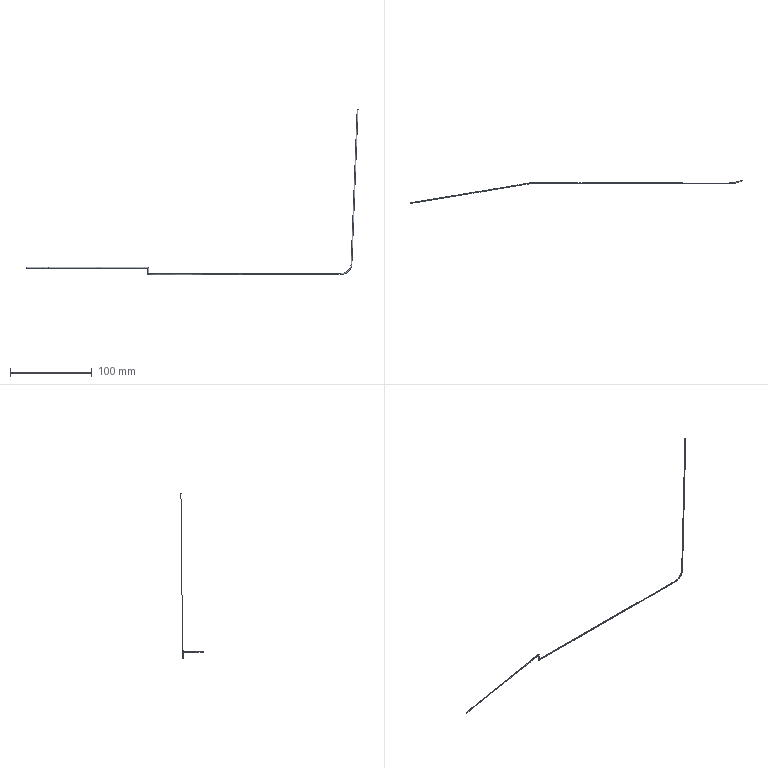Part | SolidWorks | features 3DProfileFeature 4, Sweep 1 | 1 solid | 16 faces | box 405.14 x 27.994 x 201.874 mm | volume 473.079 mm3 | spline 14 | plane 2
STEP:
#1=CARTESIAN_POINT('',(-174.988,75.046,-0.4977));
#2=VERTEX_POINT('',#1);
#3=CARTESIAN_POINT('',(-175.012,74.954,0.4977));
#4=VERTEX_POINT('',#3);
#5=CARTESIAN_POINT('',(-175.,75.,0.));
#6=DIRECTION('',(0.988,0.1497,0.03844));
#7=DIRECTION('',(0.02485,0.0916,-0.9955));
#8=AXIS2_PLACEMENT_3D('',#5,#6,#7);
#9=CIRCLE('',#8,0.5);
#10=EDGE_CURVE('',#2,#4,#9,.T.);
#11=ORIENTED_EDGE('',*,*,#10,.T.);
#12=CARTESIAN_POINT('',(-25.502,99.719,0.4977));
#13=VERTEX_POINT('',#12);
#14=CARTESIAN_POINT('',(-175.012,74.954,0.4977));
#15=CARTESIAN_POINT('',(-25.502,99.719,0.4977));
#16=B_SPLINE_CURVE_WITH_KNOTS('',1,(#14,#15),.UNSPECIFIED.,.F.,.F.,(2,2),(0.,0.9984),.UNSPECIFIED.);
#17=EDGE_CURVE('',#4,#13,#16,.T.);
#18=ORIENTED_EDGE('',*,*,#17,.T.);
#19=CARTESIAN_POINT('',(-26.498,99.641,-0.4977));
#20=VERTEX_POINT('',#19);
#21=CARTESIAN_POINT('',(-25.502,99.719,0.4977));
#22=CARTESIAN_POINT('',(-25.508,99.799,0.5047));
#23=CARTESIAN_POINT('',(-25.534,99.876,0.4915));
#24=CARTESIAN_POINT('',(-25.612,100.004,0.4354));
#25=CARTESIAN_POINT('',(-25.662,100.054,0.3942));
#26=CARTESIAN_POINT('',(-25.821,100.164,0.2555));
#27=CARTESIAN_POINT('',(-25.941,100.189,0.1418));
#28=CARTESIAN_POINT('',(-26.107,100.171,-0.02564));
#29=CARTESIAN_POINT('',(-26.162,100.156,-0.08249));
#30=CARTESIAN_POINT('',(-26.265,100.107,-0.192));
#31=CARTESIAN_POINT('',(-26.313,100.074,-0.2448));
#32=CARTESIAN_POINT('',(-26.4,99.985,-0.3451));
#33=CARTESIAN_POINT('',(-26.438,99.93,-0.3914));
#34=CARTESIAN_POINT('',(-26.49,99.798,-0.4645));
#35=CARTESIAN_POINT('',(-26.504,99.721,-0.4908));
#36=CARTESIAN_POINT('',(-26.498,99.641,-0.4977));
#37=B_SPLINE_CURVE_WITH_KNOTS('',3,(#21,#22,#23,#24,#25,#26,#27,#28,#29,#30,#31,#32,#33,#34,#35,#36),.UNSPECIFIED.,.F.,.F.,(4,2,2,2,2,2,2,4),(0.001904,0.002141,0.002379,0.002854,0.003091,0.003329,0.003566,0.003804),.UNSPECIFIED.);
#38=EDGE_CURVE('',#13,#20,#37,.T.);
#39=ORIENTED_EDGE('',*,*,#38,.T.);
#40=CARTESIAN_POINT('',(-174.988,75.046,-0.4977));
#41=CARTESIAN_POINT('',(-26.498,99.641,-0.4977));
#42=B_SPLINE_CURVE_WITH_KNOTS('',1,(#40,#41),.UNSPECIFIED.,.F.,.F.,(2,2),(0.,0.9916),.UNSPECIFIED.);
#43=EDGE_CURVE('',#2,#20,#42,.T.);
#44=ORIENTED_EDGE('',*,*,#43,.F.);
#45=EDGE_LOOP('',(#11,#18,#39,#44));
#46=FACE_OUTER_BOUND('',#45,.T.);
#47=CARTESIAN_POINT('',(-174.988,75.046,-0.4977));
#48=CARTESIAN_POINT('',(-25.244,99.849,-0.4977));
#49=CARTESIAN_POINT('',(-175.14,76.03,-0.411));
#50=CARTESIAN_POINT('',(-25.397,100.833,-0.411));
#51=CARTESIAN_POINT('',(-175.165,75.939,0.5845));
#52=CARTESIAN_POINT('',(-25.422,100.742,0.5845));
#53=CARTESIAN_POINT('',(-175.012,74.954,0.4977));
#54=CARTESIAN_POINT('',(-25.269,99.757,0.4977));
#55=CARTESIAN_POINT('',(-174.86,73.97,0.411));
#56=CARTESIAN_POINT('',(-25.117,98.773,0.411));
#57=CARTESIAN_POINT('',(-174.835,74.061,-0.5845));
#58=CARTESIAN_POINT('',(-25.092,98.864,-0.5845));
#59=CARTESIAN_POINT('',(-174.988,75.046,-0.4977));
#60=CARTESIAN_POINT('',(-25.244,99.849,-0.4977));
#61=(BOUNDED_SURFACE()B_SPLINE_SURFACE(3,1,((#47,#48),(#49,#50),(#51,#52),(#53,#54),(#55,#56),(#57,#58),(#59,#60)),.UNSPECIFIED.,.T.,.F.,.F.)B_SPLINE_SURFACE_WITH_KNOTS((4,3,4),(2,2),(0.,0.5,1.),(0.,1.),.UNSPECIFIED.)GEOMETRIC_REPRESENTATION_ITEM()RATIONAL_B_SPLINE_SURFACE(((1.,1.),(0.3333,0.3333),(0.3333,0.3333),(1.,1.),(0.3333,0.3333),(0.3333,0.3333),(1.,1.)))REPRESENTATION_ITEM('')SURFACE());
#62=ADVANCED_FACE('',(#46),#61,.T.);
#63=ORIENTED_EDGE('',*,*,#38,.F.);
#64=CARTESIAN_POINT('',(-25.502,99.719,-7.501));
#65=VERTEX_POINT('',#64);
#66=CARTESIAN_POINT('',(-25.502,99.719,0.4977));
#67=CARTESIAN_POINT('',(-25.502,99.719,-7.501));
#68=B_SPLINE_CURVE_WITH_KNOTS('',1,(#66,#67),.UNSPECIFIED.,.F.,.F.,(2,2),(0.02699,0.8746),.UNSPECIFIED.);
#69=EDGE_CURVE('',#13,#65,#68,.T.);
#70=ORIENTED_EDGE('',*,*,#69,.T.);
#71=CARTESIAN_POINT('',(-26.498,99.641,-8.499));
#72=VERTEX_POINT('',#71);
#73=CARTESIAN_POINT('',(-25.502,99.719,-7.501));
#74=CARTESIAN_POINT('',(-25.508,99.798,-7.507));
#75=CARTESIAN_POINT('',(-25.534,99.874,-7.534));
#76=CARTESIAN_POINT('',(-25.606,99.995,-7.606));
#77=CARTESIAN_POINT('',(-25.652,100.044,-7.652));
#78=CARTESIAN_POINT('',(-25.801,100.155,-7.802));
#79=CARTESIAN_POINT('',(-25.915,100.185,-7.916));
#80=CARTESIAN_POINT('',(-26.139,100.173,-8.14));
#81=CARTESIAN_POINT('',(-26.251,100.131,-8.253));
#82=CARTESIAN_POINT('',(-26.392,99.997,-8.394));
#83=CARTESIAN_POINT('',(-26.433,99.94,-8.435));
#84=CARTESIAN_POINT('',(-26.49,99.802,-8.491));
#85=CARTESIAN_POINT('',(-26.504,99.721,-8.505));
#86=CARTESIAN_POINT('',(-26.498,99.641,-8.499));
#87=B_SPLINE_CURVE_WITH_KNOTS('',3,(#73,#74,#75,#76,#77,#78,#79,#80,#81,#82,#83,#84,#85,#86),.UNSPECIFIED.,.F.,.F.,(4,2,2,2,2,2,4),(0.001903,0.002141,0.002379,0.002855,0.00333,0.003568,0.003806),.UNSPECIFIED.);
#88=EDGE_CURVE('',#65,#72,#87,.T.);
#89=ORIENTED_EDGE('',*,*,#88,.T.);
#90=CARTESIAN_POINT('',(-26.498,99.641,-0.4977));
#91=CARTESIAN_POINT('',(-26.498,99.641,-8.499));
#92=B_SPLINE_CURVE_WITH_KNOTS('',1,(#90,#91),.UNSPECIFIED.,.F.,.F.,(2,2),(0.1283,0.9762),.UNSPECIFIED.);
#93=EDGE_CURVE('',#20,#72,#92,.T.);
#94=ORIENTED_EDGE('',*,*,#93,.F.);
#95=EDGE_LOOP('',(#63,#70,#89,#94));
#96=FACE_OUTER_BOUND('',#95,.T.);
#97=CARTESIAN_POINT('',(-26.498,99.641,0.7129));
#98=CARTESIAN_POINT('',(-26.498,99.641,-8.724));
#99=CARTESIAN_POINT('',(-26.575,100.638,0.7026));
#100=CARTESIAN_POINT('',(-26.575,100.638,-8.734));
#101=CARTESIAN_POINT('',(-25.579,100.716,0.742));
#102=CARTESIAN_POINT('',(-25.579,100.716,-8.694));
#103=CARTESIAN_POINT('',(-25.502,99.719,0.7524));
#104=CARTESIAN_POINT('',(-25.502,99.719,-8.684));
#105=CARTESIAN_POINT('',(-25.425,98.722,0.7628));
#106=CARTESIAN_POINT('',(-25.425,98.722,-8.674));
#107=CARTESIAN_POINT('',(-26.421,98.644,0.7233));
#108=CARTESIAN_POINT('',(-26.421,98.644,-8.713));
#109=CARTESIAN_POINT('',(-26.498,99.641,0.7129));
#110=CARTESIAN_POINT('',(-26.498,99.641,-8.724));
#111=(BOUNDED_SURFACE()B_SPLINE_SURFACE(3,1,((#97,#98),(#99,#100),(#101,#102),(#103,#104),(#105,#106),(#107,#108),(#109,#110)),.UNSPECIFIED.,.T.,.F.,.F.)B_SPLINE_SURFACE_WITH_KNOTS((4,3,4),(2,2),(0.,0.5,1.),(0.,1.),.UNSPECIFIED.)GEOMETRIC_REPRESENTATION_ITEM()RATIONAL_B_SPLINE_SURFACE(((1.,1.),(0.3333,0.3333),(0.3333,0.3333),(1.,1.),(0.3333,0.3333),(0.3333,0.3333),(1.,1.)))REPRESENTATION_ITEM('')SURFACE());
#112=ADVANCED_FACE('',(#96),#111,.T.);
#113=CARTESIAN_POINT('',(222.574,100.029,3.873));
#114=VERTEX_POINT('',#113);
#115=CARTESIAN_POINT('',(221.574,100.029,3.873));
#116=VERTEX_POINT('',#115);
#117=CARTESIAN_POINT('',(222.074,100.029,3.873));
#118=DIRECTION('',(0.,0.,1.));
#119=DIRECTION('',(1.,0.,0.));
#120=AXIS2_PLACEMENT_3D('',#117,#118,#119);
#121=CIRCLE('',#120,0.5);
#122=EDGE_CURVE('',#114,#116,#121,.T.);
#123=ORIENTED_EDGE('',*,*,#122,.T.);
#124=CARTESIAN_POINT('',(229.063,102.,193.373));
#125=VERTEX_POINT('',#124);
#126=CARTESIAN_POINT('',(221.574,100.029,3.873));
#127=CARTESIAN_POINT('',(229.063,102.,193.373));
#128=B_SPLINE_CURVE_WITH_KNOTS('',1,(#126,#127),.UNSPECIFIED.,.F.,.F.,(2,2),(0.,1.),.UNSPECIFIED.);
#129=EDGE_CURVE('',#116,#125,#128,.T.);
#130=ORIENTED_EDGE('',*,*,#129,.T.);
#131=CARTESIAN_POINT('',(230.063,102.,193.373));
#132=VERTEX_POINT('',#131);
#133=CARTESIAN_POINT('',(229.563,102.,193.373));
#134=DIRECTION('',(0.,0.,1.));
#135=DIRECTION('',(1.,0.,0.));
#136=AXIS2_PLACEMENT_3D('',#133,#134,#135);
#137=CIRCLE('',#136,0.5);
#138=EDGE_CURVE('',#132,#125,#137,.T.);
#139=ORIENTED_EDGE('',*,*,#138,.F.);
#140=CARTESIAN_POINT('',(222.574,100.029,3.873));
#141=CARTESIAN_POINT('',(230.063,102.,193.373));
#142=B_SPLINE_CURVE_WITH_KNOTS('',1,(#140,#141),.UNSPECIFIED.,.F.,.F.,(2,2),(0.,1.),.UNSPECIFIED.);
#143=EDGE_CURVE('',#114,#132,#142,.T.);
#144=ORIENTED_EDGE('',*,*,#143,.F.);
#145=EDGE_LOOP('',(#123,#130,#139,#144));
#146=FACE_OUTER_BOUND('',#145,.T.);
#147=CARTESIAN_POINT('',(222.574,100.029,3.873));
#148=CARTESIAN_POINT('',(230.063,102.,193.373));
#149=CARTESIAN_POINT('',(222.574,101.029,3.873));
#150=CARTESIAN_POINT('',(230.063,103.,193.373));
#151=CARTESIAN_POINT('',(221.574,101.029,3.873));
#152=CARTESIAN_POINT('',(229.063,103.,193.373));
#153=CARTESIAN_POINT('',(221.574,100.029,3.873));
#154=CARTESIAN_POINT('',(229.063,102.,193.373));
#155=CARTESIAN_POINT('',(221.574,99.029,3.873));
#156=CARTESIAN_POINT('',(229.063,101.,193.373));
#157=CARTESIAN_POINT('',(222.574,99.029,3.873));
#158=CARTESIAN_POINT('',(230.063,101.,193.373));
#159=CARTESIAN_POINT('',(222.574,100.029,3.873));
#160=CARTESIAN_POINT('',(230.063,102.,193.373));
#161=(BOUNDED_SURFACE()B_SPLINE_SURFACE(3,1,((#147,#148),(#149,#150),(#151,#152),(#153,#154),(#155,#156),(#157,#158),(#159,#160)),.UNSPECIFIED.,.T.,.F.,.T.)B_SPLINE_SURFACE_WITH_KNOTS((4,3,4),(2,2),(0.,0.5,1.),(0.,1.),.UNSPECIFIED.)GEOMETRIC_REPRESENTATION_ITEM()RATIONAL_B_SPLINE_SURFACE(((1.,1.),(0.3333,0.3333),(0.3333,0.3333),(1.,1.),(0.3333,0.3333),(0.3333,0.3333),(1.,1.)))REPRESENTATION_ITEM('')SURFACE());
#162=ADVANCED_FACE('',(#146),#161,.T.);
#163=CARTESIAN_POINT('',(220.924,99.723,-1.425));
#164=VERTEX_POINT('',#163);
#165=CARTESIAN_POINT('',(220.06,99.749,-0.9214));
#166=VERTEX_POINT('',#165);
#167=CARTESIAN_POINT('',(220.492,99.736,-1.173));
#168=DIRECTION('',(0.5033,0.08685,0.8598));
#169=DIRECTION('',(0.8639,-0.02541,-0.5031));
#170=AXIS2_PLACEMENT_3D('',#167,#168,#169);
#171=CIRCLE('',#170,0.5);
#172=EDGE_CURVE('',#164,#166,#171,.T.);
#173=ORIENTED_EDGE('',*,*,#172,.T.);
#174=CARTESIAN_POINT('',(220.06,99.749,-0.9214));
#175=CARTESIAN_POINT('',(220.985,99.915,0.5179));
#176=CARTESIAN_POINT('',(221.502,100.01,2.155));
#177=CARTESIAN_POINT('',(221.574,100.029,3.873));
#178=(BOUNDED_CURVE()B_SPLINE_CURVE(3,(#174,#175,#176,#177),.UNSPECIFIED.,.F.,.F.)B_SPLINE_CURVE_WITH_KNOTS((4,4),(0.,1.),.UNSPECIFIED.)CURVE()GEOMETRIC_REPRESENTATION_ITEM()RATIONAL_B_SPLINE_CURVE((1.,0.9762,0.9762,1.))REPRESENTATION_ITEM(''));
#179=EDGE_CURVE('',#166,#116,#178,.T.);
#180=ORIENTED_EDGE('',*,*,#179,.T.);
#181=ORIENTED_EDGE('',*,*,#122,.F.);
#182=CARTESIAN_POINT('',(220.924,99.723,-1.425));
#183=CARTESIAN_POINT('',(221.939,99.905,0.168));
#184=CARTESIAN_POINT('',(222.502,100.009,1.977));
#185=CARTESIAN_POINT('',(222.574,100.029,3.873));
#186=(BOUNDED_CURVE()B_SPLINE_CURVE(3,(#182,#183,#184,#185),.UNSPECIFIED.,.F.,.T.)B_SPLINE_CURVE_WITH_KNOTS((4,4),(0.,1.),.UNSPECIFIED.)CURVE()GEOMETRIC_REPRESENTATION_ITEM()RATIONAL_B_SPLINE_CURVE((1.,0.9762,0.9762,1.))REPRESENTATION_ITEM(''));
#187=EDGE_CURVE('',#164,#114,#186,.T.);
#188=ORIENTED_EDGE('',*,*,#187,.F.);
#189=EDGE_LOOP('',(#173,#180,#181,#188));
#190=FACE_OUTER_BOUND('',#189,.T.);
#191=CARTESIAN_POINT('',(220.924,99.723,-1.425));
#192=CARTESIAN_POINT('',(221.939,99.905,0.168));
#193=CARTESIAN_POINT('',(222.502,100.009,1.977));
#194=CARTESIAN_POINT('',(222.574,100.029,3.873));
#195=CARTESIAN_POINT('',(220.902,100.719,-1.512));
#196=CARTESIAN_POINT('',(221.932,100.904,0.107));
#197=CARTESIAN_POINT('',(222.503,101.009,1.946));
#198=CARTESIAN_POINT('',(222.574,101.029,3.873));
#199=CARTESIAN_POINT('',(220.038,100.745,-1.009));
#200=CARTESIAN_POINT('',(220.979,100.913,0.457));
#201=CARTESIAN_POINT('',(221.503,101.01,2.124));
#202=CARTESIAN_POINT('',(221.574,101.029,3.873));
#203=CARTESIAN_POINT('',(220.06,99.749,-0.9214));
#204=CARTESIAN_POINT('',(220.985,99.915,0.5179));
#205=CARTESIAN_POINT('',(221.502,100.01,2.155));
#206=CARTESIAN_POINT('',(221.574,100.029,3.873));
#207=CARTESIAN_POINT('',(220.082,98.753,-0.8336));
#208=CARTESIAN_POINT('',(220.992,98.916,0.5788));
#209=CARTESIAN_POINT('',(221.502,99.01,2.186));
#210=CARTESIAN_POINT('',(221.574,99.029,3.873));
#211=CARTESIAN_POINT('',(220.945,98.727,-1.337));
#212=CARTESIAN_POINT('',(221.946,98.907,0.2289));
#213=CARTESIAN_POINT('',(222.502,99.009,2.008));
#214=CARTESIAN_POINT('',(222.574,99.029,3.873));
#215=CARTESIAN_POINT('',(220.924,99.723,-1.425));
#216=CARTESIAN_POINT('',(221.939,99.905,0.168));
#217=CARTESIAN_POINT('',(222.502,100.009,1.977));
#218=CARTESIAN_POINT('',(222.574,100.029,3.873));
#219=(BOUNDED_SURFACE()B_SPLINE_SURFACE(3,3,((#191,#192,#193,#194),(#195,#196,#197,#198),(#199,#200,#201,#202),(#203,#204,#205,#206),(#207,#208,#209,#210),(#211,#212,#213,#214),(#215,#216,#217,#218)),.UNSPECIFIED.,.T.,.F.,.F.)B_SPLINE_SURFACE_WITH_KNOTS((4,3,4),(4,4),(0.,0.5,1.),(0.,1.),.UNSPECIFIED.)GEOMETRIC_REPRESENTATION_ITEM()RATIONAL_B_SPLINE_SURFACE(((1.,0.9762,0.9762,1.),(0.3333,0.3254,0.3254,0.3333),(0.3333,0.3254,0.3254,0.3333),(1.,0.9762,0.9762,1.),(0.3333,0.3254,0.3254,0.3333),(0.3333,0.3254,0.3254,0.3333),(1.,0.9762,0.9762,1.)))REPRESENTATION_ITEM('')SURFACE());
#220=ADVANCED_FACE('',(#190),#219,.T.);
#221=CARTESIAN_POINT('',(220.679,99.68,-1.806));
#222=VERTEX_POINT('',#221);
#223=CARTESIAN_POINT('',(219.815,99.705,-1.303));
#224=VERTEX_POINT('',#223);
#225=CARTESIAN_POINT('',(220.247,99.692,-1.555));
#226=DIRECTION('',(0.5033,0.08685,0.8598));
#227=DIRECTION('',(0.8639,-0.02541,-0.5031));
#228=AXIS2_PLACEMENT_3D('',#225,#226,#227);
#229=CIRCLE('',#228,0.5);
#230=EDGE_CURVE('',#222,#224,#229,.T.);
#231=ORIENTED_EDGE('',*,*,#230,.T.);
#232=CARTESIAN_POINT('',(219.815,99.705,-1.303));
#233=CARTESIAN_POINT('',(220.06,99.749,-0.9214));
#234=B_SPLINE_CURVE_WITH_KNOTS('',1,(#232,#233),.UNSPECIFIED.,.F.,.F.,(2,2),(0.,1.),.UNSPECIFIED.);
#235=EDGE_CURVE('',#224,#166,#234,.T.);
#236=ORIENTED_EDGE('',*,*,#235,.T.);
#237=ORIENTED_EDGE('',*,*,#172,.F.);
#238=CARTESIAN_POINT('',(220.679,99.68,-1.806));
#239=CARTESIAN_POINT('',(220.924,99.723,-1.425));
#240=B_SPLINE_CURVE_WITH_KNOTS('',1,(#238,#239),.UNSPECIFIED.,.F.,.F.,(2,2),(0.,1.),.UNSPECIFIED.);
#241=EDGE_CURVE('',#222,#164,#240,.T.);
#242=ORIENTED_EDGE('',*,*,#241,.F.);
#243=EDGE_LOOP('',(#231,#236,#237,#242));
#244=FACE_OUTER_BOUND('',#243,.T.);
#245=CARTESIAN_POINT('',(220.679,99.68,-1.806));
#246=CARTESIAN_POINT('',(220.924,99.723,-1.425));
#247=CARTESIAN_POINT('',(220.657,100.675,-1.894));
#248=CARTESIAN_POINT('',(220.902,100.719,-1.512));
#249=CARTESIAN_POINT('',(219.793,100.701,-1.391));
#250=CARTESIAN_POINT('',(220.038,100.745,-1.009));
#251=CARTESIAN_POINT('',(219.815,99.705,-1.303));
#252=CARTESIAN_POINT('',(220.06,99.749,-0.9214));
#253=CARTESIAN_POINT('',(219.837,98.709,-1.215));
#254=CARTESIAN_POINT('',(220.082,98.753,-0.8336));
#255=CARTESIAN_POINT('',(220.701,98.684,-1.718));
#256=CARTESIAN_POINT('',(220.945,98.727,-1.337));
#257=CARTESIAN_POINT('',(220.679,99.68,-1.806));
#258=CARTESIAN_POINT('',(220.924,99.723,-1.425));
#259=(BOUNDED_SURFACE()B_SPLINE_SURFACE(3,1,((#245,#246),(#247,#248),(#249,#250),(#251,#252),(#253,#254),(#255,#256),(#257,#258)),.UNSPECIFIED.,.T.,.F.,.T.)B_SPLINE_SURFACE_WITH_KNOTS((4,3,4),(2,2),(0.,0.5,1.),(0.,1.),.UNSPECIFIED.)GEOMETRIC_REPRESENTATION_ITEM()RATIONAL_B_SPLINE_SURFACE(((1.,1.),(0.3333,0.3333),(0.3333,0.3333),(1.,1.),(0.3333,0.3333),(0.3333,0.3333),(1.,1.)))REPRESENTATION_ITEM('')SURFACE());
#260=ADVANCED_FACE('',(#244),#259,.T.);
#261=CARTESIAN_POINT('',(209.32,98.987,-8.038));
#262=VERTEX_POINT('',#261);
#263=CARTESIAN_POINT('',(209.279,99.067,-7.043));
#264=VERTEX_POINT('',#263);
#265=CARTESIAN_POINT('',(209.299,99.027,-7.541));
#266=DIRECTION('',(0.9991,-0.009968,0.04215));
#267=DIRECTION('',(0.04121,-0.0804,-0.9959));
#268=AXIS2_PLACEMENT_3D('',#265,#266,#267);
#269=CIRCLE('',#268,0.5);
#270=EDGE_CURVE('',#262,#264,#269,.T.);
#271=ORIENTED_EDGE('',*,*,#270,.T.);
#272=CARTESIAN_POINT('',(209.279,99.067,-7.043));
#273=CARTESIAN_POINT('',(213.642,99.055,-7.041));
#274=CARTESIAN_POINT('',(217.468,99.286,-4.957));
#275=CARTESIAN_POINT('',(219.815,99.705,-1.303));
#276=(BOUNDED_CURVE()B_SPLINE_CURVE(3,(#272,#273,#274,#275),.UNSPECIFIED.,.F.,.T.)B_SPLINE_CURVE_WITH_KNOTS((4,4),(0.,1.),.UNSPECIFIED.)CURVE()GEOMETRIC_REPRESENTATION_ITEM()RATIONAL_B_SPLINE_CURVE((1.,0.918,0.918,1.))REPRESENTATION_ITEM(''));
#277=EDGE_CURVE('',#264,#224,#276,.T.);
#278=ORIENTED_EDGE('',*,*,#277,.T.);
#279=ORIENTED_EDGE('',*,*,#230,.F.);
#280=CARTESIAN_POINT('',(209.32,98.987,-8.038));
#281=CARTESIAN_POINT('',(214.031,98.975,-8.022));
#282=CARTESIAN_POINT('',(218.156,99.226,-5.759));
#283=CARTESIAN_POINT('',(220.679,99.68,-1.806));
#284=(BOUNDED_CURVE()B_SPLINE_CURVE(3,(#280,#281,#282,#283),.UNSPECIFIED.,.F.,.T.)B_SPLINE_CURVE_WITH_KNOTS((4,4),(0.,1.),.UNSPECIFIED.)CURVE()GEOMETRIC_REPRESENTATION_ITEM()RATIONAL_B_SPLINE_CURVE((1.,0.918,0.918,1.))REPRESENTATION_ITEM(''));
#285=EDGE_CURVE('',#262,#222,#284,.T.);
#286=ORIENTED_EDGE('',*,*,#285,.F.);
#287=EDGE_LOOP('',(#271,#278,#279,#286));
#288=FACE_OUTER_BOUND('',#287,.T.);
#289=CARTESIAN_POINT('',(209.32,98.987,-8.038));
#290=CARTESIAN_POINT('',(214.031,98.975,-8.022));
#291=CARTESIAN_POINT('',(218.156,99.226,-5.759));
#292=CARTESIAN_POINT('',(220.679,99.68,-1.806));
#293=CARTESIAN_POINT('',(209.333,99.984,-8.118));
#294=CARTESIAN_POINT('',(214.032,99.972,-8.099));
#295=CARTESIAN_POINT('',(218.144,100.223,-5.839));
#296=CARTESIAN_POINT('',(220.657,100.675,-1.894));
#297=CARTESIAN_POINT('',(209.292,100.064,-7.123));
#298=CARTESIAN_POINT('',(213.642,100.052,-7.117));
#299=CARTESIAN_POINT('',(217.456,100.283,-5.036));
#300=CARTESIAN_POINT('',(219.793,100.701,-1.391));
#301=CARTESIAN_POINT('',(209.279,99.067,-7.043));
#302=CARTESIAN_POINT('',(213.642,99.055,-7.041));
#303=CARTESIAN_POINT('',(217.468,99.286,-4.957));
#304=CARTESIAN_POINT('',(219.815,99.705,-1.303));
#305=CARTESIAN_POINT('',(209.265,98.071,-6.963));
#306=CARTESIAN_POINT('',(213.641,98.057,-6.965));
#307=CARTESIAN_POINT('',(217.48,98.289,-4.878));
#308=CARTESIAN_POINT('',(219.837,98.709,-1.215));
#309=CARTESIAN_POINT('',(209.307,97.99,-7.959));
#310=CARTESIAN_POINT('',(214.031,97.978,-7.946));
#311=CARTESIAN_POINT('',(218.168,98.229,-5.68));
#312=CARTESIAN_POINT('',(220.701,98.684,-1.718));
#313=CARTESIAN_POINT('',(209.32,98.987,-8.038));
#314=CARTESIAN_POINT('',(214.031,98.975,-8.022));
#315=CARTESIAN_POINT('',(218.156,99.226,-5.759));
#316=CARTESIAN_POINT('',(220.679,99.68,-1.806));
#317=(BOUNDED_SURFACE()B_SPLINE_SURFACE(3,3,((#289,#290,#291,#292),(#293,#294,#295,#296),(#297,#298,#299,#300),(#301,#302,#303,#304),(#305,#306,#307,#308),(#309,#310,#311,#312),(#313,#314,#315,#316)),.UNSPECIFIED.,.T.,.F.,.F.)B_SPLINE_SURFACE_WITH_KNOTS((4,3,4),(4,4),(0.,0.5,1.),(0.,1.),.UNSPECIFIED.)GEOMETRIC_REPRESENTATION_ITEM()RATIONAL_B_SPLINE_SURFACE(((1.,0.918,0.918,1.),(0.3333,0.306,0.306,0.3333),(0.3333,0.306,0.306,0.3333),(1.,0.918,0.918,1.),(0.3333,0.306,0.306,0.3333),(0.3333,0.306,0.306,0.3333),(1.,0.918,0.918,1.)))REPRESENTATION_ITEM('')SURFACE());
#318=ADVANCED_FACE('',(#288),#317,.T.);
#319=ORIENTED_EDGE('',*,*,#88,.F.);
#320=CARTESIAN_POINT('',(-25.502,99.719,-7.501));
#321=CARTESIAN_POINT('',(209.279,99.067,-7.043));
#322=B_SPLINE_CURVE_WITH_KNOTS('',1,(#320,#321),.UNSPECIFIED.,.F.,.F.,(2,2),(0.00546,1.),.UNSPECIFIED.);
#323=EDGE_CURVE('',#65,#264,#322,.T.);
#324=ORIENTED_EDGE('',*,*,#323,.T.);
#325=ORIENTED_EDGE('',*,*,#270,.F.);
#326=CARTESIAN_POINT('',(-26.498,99.641,-8.499));
#327=CARTESIAN_POINT('',(209.32,98.987,-8.038));
#328=B_SPLINE_CURVE_WITH_KNOTS('',1,(#326,#327),.UNSPECIFIED.,.F.,.F.,(2,2),(0.001065,1.),.UNSPECIFIED.);
#329=EDGE_CURVE('',#72,#262,#328,.T.);
#330=ORIENTED_EDGE('',*,*,#329,.F.);
#331=EDGE_LOOP('',(#319,#324,#325,#330));
#332=FACE_OUTER_BOUND('',#331,.T.);
#333=CARTESIAN_POINT('',(-26.75,99.642,-8.499));
#334=CARTESIAN_POINT('',(209.32,98.987,-8.038));
#335=CARTESIAN_POINT('',(-26.736,100.639,-8.579));
#336=CARTESIAN_POINT('',(209.333,99.984,-8.118));
#337=CARTESIAN_POINT('',(-26.777,100.719,-7.583));
#338=CARTESIAN_POINT('',(209.292,100.064,-7.123));
#339=CARTESIAN_POINT('',(-26.791,99.722,-7.504));
#340=CARTESIAN_POINT('',(209.279,99.067,-7.043));
#341=CARTESIAN_POINT('',(-26.804,98.726,-7.424));
#342=CARTESIAN_POINT('',(209.265,98.071,-6.963));
#343=CARTESIAN_POINT('',(-26.763,98.645,-8.42));
#344=CARTESIAN_POINT('',(209.307,97.99,-7.959));
#345=CARTESIAN_POINT('',(-26.75,99.642,-8.499));
#346=CARTESIAN_POINT('',(209.32,98.987,-8.038));
#347=(BOUNDED_SURFACE()B_SPLINE_SURFACE(3,1,((#333,#334),(#335,#336),(#337,#338),(#339,#340),(#341,#342),(#343,#344),(#345,#346)),.UNSPECIFIED.,.T.,.F.,.T.)B_SPLINE_SURFACE_WITH_KNOTS((4,3,4),(2,2),(0.,0.5,1.),(0.,1.),.UNSPECIFIED.)GEOMETRIC_REPRESENTATION_ITEM()RATIONAL_B_SPLINE_SURFACE(((1.,1.),(0.3333,0.3333),(0.3333,0.3333),(1.,1.),(0.3333,0.3333),(0.3333,0.3333),(1.,1.)))REPRESENTATION_ITEM('')SURFACE());
#348=ADVANCED_FACE('',(#332),#347,.T.);
#349=ORIENTED_EDGE('',*,*,#17,.F.);
#350=CARTESIAN_POINT('',(-175.,75.,0.));
#351=DIRECTION('',(0.988,0.1497,0.03844));
#352=DIRECTION('',(0.02485,0.0916,-0.9955));
#353=AXIS2_PLACEMENT_3D('',#350,#351,#352);
#354=CIRCLE('',#353,0.5);
#355=EDGE_CURVE('',#4,#2,#354,.T.);
#356=ORIENTED_EDGE('',*,*,#355,.T.);
#357=ORIENTED_EDGE('',*,*,#43,.T.);
#358=CARTESIAN_POINT('',(-26.498,99.641,-0.4977));
#359=CARTESIAN_POINT('',(-26.492,99.561,-0.5047));
#360=CARTESIAN_POINT('',(-26.466,99.484,-0.4915));
#361=CARTESIAN_POINT('',(-26.388,99.356,-0.4355));
#362=CARTESIAN_POINT('',(-26.338,99.306,-0.3943));
#363=CARTESIAN_POINT('',(-26.179,99.196,-0.2555));
#364=CARTESIAN_POINT('',(-26.059,99.171,-0.1418));
#365=CARTESIAN_POINT('',(-25.893,99.189,0.02565));
#366=CARTESIAN_POINT('',(-25.838,99.204,0.08248));
#367=CARTESIAN_POINT('',(-25.735,99.253,0.1921));
#368=CARTESIAN_POINT('',(-25.687,99.286,0.2448));
#369=CARTESIAN_POINT('',(-25.6,99.375,0.3451));
#370=CARTESIAN_POINT('',(-25.562,99.43,0.3914));
#371=CARTESIAN_POINT('',(-25.509,99.562,0.4646));
#372=CARTESIAN_POINT('',(-25.496,99.639,0.4908));
#373=CARTESIAN_POINT('',(-25.502,99.719,0.4977));
#374=B_SPLINE_CURVE_WITH_KNOTS('',3,(#358,#359,#360,#361,#362,#363,#364,#365,#366,#367,#368,#369,#370,#371,#372,#373),.UNSPECIFIED.,.F.,.F.,(4,2,2,2,2,2,2,4),(0.,0.000238,0.0004759,0.0009518,0.00119,0.001428,0.001666,0.001904),.UNSPECIFIED.);
#375=EDGE_CURVE('',#20,#13,#374,.T.);
#376=ORIENTED_EDGE('',*,*,#375,.T.);
#377=EDGE_LOOP('',(#349,#356,#357,#376));
#378=FACE_OUTER_BOUND('',#377,.T.);
#379=CARTESIAN_POINT('',(-174.988,75.046,-0.4977));
#380=CARTESIAN_POINT('',(-25.244,99.849,-0.4977));
#381=CARTESIAN_POINT('',(-175.14,76.03,-0.411));
#382=CARTESIAN_POINT('',(-25.397,100.833,-0.411));
#383=CARTESIAN_POINT('',(-175.165,75.939,0.5845));
#384=CARTESIAN_POINT('',(-25.422,100.742,0.5845));
#385=CARTESIAN_POINT('',(-175.012,74.954,0.4977));
#386=CARTESIAN_POINT('',(-25.269,99.757,0.4977));
#387=CARTESIAN_POINT('',(-174.86,73.97,0.411));
#388=CARTESIAN_POINT('',(-25.117,98.773,0.411));
#389=CARTESIAN_POINT('',(-174.835,74.061,-0.5845));
#390=CARTESIAN_POINT('',(-25.092,98.864,-0.5845));
#391=CARTESIAN_POINT('',(-174.988,75.046,-0.4977));
#392=CARTESIAN_POINT('',(-25.244,99.849,-0.4977));
#393=(BOUNDED_SURFACE()B_SPLINE_SURFACE(3,1,((#379,#380),(#381,#382),(#383,#384),(#385,#386),(#387,#388),(#389,#390),(#391,#392)),.UNSPECIFIED.,.T.,.F.,.T.)B_SPLINE_SURFACE_WITH_KNOTS((4,3,4),(2,2),(0.,0.5,1.),(0.,1.),.UNSPECIFIED.)GEOMETRIC_REPRESENTATION_ITEM()RATIONAL_B_SPLINE_SURFACE(((1.,1.),(0.3333,0.3333),(0.3333,0.3333),(1.,1.),(0.3333,0.3333),(0.3333,0.3333),(1.,1.)))REPRESENTATION_ITEM('')SURFACE());
#394=ADVANCED_FACE('',(#378),#393,.T.);
#395=ORIENTED_EDGE('',*,*,#69,.F.);
#396=ORIENTED_EDGE('',*,*,#375,.F.);
#397=ORIENTED_EDGE('',*,*,#93,.T.);
#398=CARTESIAN_POINT('',(-26.498,99.641,-8.499));
#399=CARTESIAN_POINT('',(-26.492,99.561,-8.493));
#400=CARTESIAN_POINT('',(-26.466,99.487,-8.467));
#401=CARTESIAN_POINT('',(-26.394,99.365,-8.394));
#402=CARTESIAN_POINT('',(-26.349,99.316,-8.348));
#403=CARTESIAN_POINT('',(-26.199,99.205,-8.198));
#404=CARTESIAN_POINT('',(-26.085,99.175,-8.084));
#405=CARTESIAN_POINT('',(-25.862,99.187,-7.86));
#406=CARTESIAN_POINT('',(-25.748,99.23,-7.746));
#407=CARTESIAN_POINT('',(-25.609,99.363,-7.607));
#408=CARTESIAN_POINT('',(-25.567,99.42,-7.565));
#409=CARTESIAN_POINT('',(-25.51,99.558,-7.509));
#410=CARTESIAN_POINT('',(-25.496,99.64,-7.495));
#411=CARTESIAN_POINT('',(-25.502,99.719,-7.501));
#412=B_SPLINE_CURVE_WITH_KNOTS('',3,(#398,#399,#400,#401,#402,#403,#404,#405,#406,#407,#408,#409,#410,#411),.UNSPECIFIED.,.F.,.F.,(4,2,2,2,2,2,4),(0.,0.0002379,0.0004757,0.0009515,0.001427,0.001665,0.001903),.UNSPECIFIED.);
#413=EDGE_CURVE('',#72,#65,#412,.T.);
#414=ORIENTED_EDGE('',*,*,#413,.T.);
#415=EDGE_LOOP('',(#395,#396,#397,#414));
#416=FACE_OUTER_BOUND('',#415,.T.);
#417=CARTESIAN_POINT('',(-26.498,99.641,0.7129));
#418=CARTESIAN_POINT('',(-26.498,99.641,-8.724));
#419=CARTESIAN_POINT('',(-26.575,100.638,0.7026));
#420=CARTESIAN_POINT('',(-26.575,100.638,-8.734));
#421=CARTESIAN_POINT('',(-25.579,100.716,0.742));
#422=CARTESIAN_POINT('',(-25.579,100.716,-8.694));
#423=CARTESIAN_POINT('',(-25.502,99.719,0.7524));
#424=CARTESIAN_POINT('',(-25.502,99.719,-8.684));
#425=CARTESIAN_POINT('',(-25.425,98.722,0.7628));
#426=CARTESIAN_POINT('',(-25.425,98.722,-8.674));
#427=CARTESIAN_POINT('',(-26.421,98.644,0.7233));
#428=CARTESIAN_POINT('',(-26.421,98.644,-8.713));
#429=CARTESIAN_POINT('',(-26.498,99.641,0.7129));
#430=CARTESIAN_POINT('',(-26.498,99.641,-8.724));
#431=(BOUNDED_SURFACE()B_SPLINE_SURFACE(3,1,((#417,#418),(#419,#420),(#421,#422),(#423,#424),(#425,#426),(#427,#428),(#429,#430)),.UNSPECIFIED.,.T.,.F.,.F.)B_SPLINE_SURFACE_WITH_KNOTS((4,3,4),(2,2),(0.,0.5,1.),(0.,1.),.UNSPECIFIED.)GEOMETRIC_REPRESENTATION_ITEM()RATIONAL_B_SPLINE_SURFACE(((1.,1.),(0.3333,0.3333),(0.3333,0.3333),(1.,1.),(0.3333,0.3333),(0.3333,0.3333),(1.,1.)))REPRESENTATION_ITEM('')SURFACE());
#432=ADVANCED_FACE('',(#416),#431,.T.);
#433=ORIENTED_EDGE('',*,*,#129,.F.);
#434=CARTESIAN_POINT('',(222.074,100.029,3.873));
#435=DIRECTION('',(0.,0.,1.));
#436=DIRECTION('',(1.,0.,0.));
#437=AXIS2_PLACEMENT_3D('',#434,#435,#436);
#438=CIRCLE('',#437,0.5);
#439=EDGE_CURVE('',#116,#114,#438,.T.);
#440=ORIENTED_EDGE('',*,*,#439,.T.);
#441=ORIENTED_EDGE('',*,*,#143,.T.);
#442=CARTESIAN_POINT('',(229.563,102.,193.373));
#443=DIRECTION('',(0.,0.,1.));
#444=DIRECTION('',(1.,0.,0.));
#445=AXIS2_PLACEMENT_3D('',#442,#443,#444);
#446=CIRCLE('',#445,0.5);
#447=EDGE_CURVE('',#125,#132,#446,.T.);
#448=ORIENTED_EDGE('',*,*,#447,.F.);
#449=EDGE_LOOP('',(#433,#440,#441,#448));
#450=FACE_OUTER_BOUND('',#449,.T.);
#451=CARTESIAN_POINT('',(222.574,100.029,3.873));
#452=CARTESIAN_POINT('',(230.063,102.,193.373));
#453=CARTESIAN_POINT('',(222.574,101.029,3.873));
#454=CARTESIAN_POINT('',(230.063,103.,193.373));
#455=CARTESIAN_POINT('',(221.574,101.029,3.873));
#456=CARTESIAN_POINT('',(229.063,103.,193.373));
#457=CARTESIAN_POINT('',(221.574,100.029,3.873));
#458=CARTESIAN_POINT('',(229.063,102.,193.373));
#459=CARTESIAN_POINT('',(221.574,99.029,3.873));
#460=CARTESIAN_POINT('',(229.063,101.,193.373));
#461=CARTESIAN_POINT('',(222.574,99.029,3.873));
#462=CARTESIAN_POINT('',(230.063,101.,193.373));
#463=CARTESIAN_POINT('',(222.574,100.029,3.873));
#464=CARTESIAN_POINT('',(230.063,102.,193.373));
#465=(BOUNDED_SURFACE()B_SPLINE_SURFACE(3,1,((#451,#452),(#453,#454),(#455,#456),(#457,#458),(#459,#460),(#461,#462),(#463,#464)),.UNSPECIFIED.,.T.,.F.,.F.)B_SPLINE_SURFACE_WITH_KNOTS((4,3,4),(2,2),(0.,0.5,1.),(0.,1.),.UNSPECIFIED.)GEOMETRIC_REPRESENTATION_ITEM()RATIONAL_B_SPLINE_SURFACE(((1.,1.),(0.3333,0.3333),(0.3333,0.3333),(1.,1.),(0.3333,0.3333),(0.3333,0.3333),(1.,1.)))REPRESENTATION_ITEM('')SURFACE());
#466=ADVANCED_FACE('',(#450),#465,.T.);
#467=ORIENTED_EDGE('',*,*,#179,.F.);
#468=CARTESIAN_POINT('',(220.492,99.736,-1.173));
#469=DIRECTION('',(0.5033,0.08685,0.8598));
#470=DIRECTION('',(0.8639,-0.02541,-0.5031));
#471=AXIS2_PLACEMENT_3D('',#468,#469,#470);
#472=CIRCLE('',#471,0.5);
#473=EDGE_CURVE('',#166,#164,#472,.T.);
#474=ORIENTED_EDGE('',*,*,#473,.T.);
#475=ORIENTED_EDGE('',*,*,#187,.T.);
#476=ORIENTED_EDGE('',*,*,#439,.F.);
#477=EDGE_LOOP('',(#467,#474,#475,#476));
#478=FACE_OUTER_BOUND('',#477,.T.);
#479=CARTESIAN_POINT('',(220.924,99.723,-1.425));
#480=CARTESIAN_POINT('',(221.939,99.905,0.168));
#481=CARTESIAN_POINT('',(222.502,100.009,1.977));
#482=CARTESIAN_POINT('',(222.574,100.029,3.873));
#483=CARTESIAN_POINT('',(220.902,100.719,-1.512));
#484=CARTESIAN_POINT('',(221.932,100.904,0.107));
#485=CARTESIAN_POINT('',(222.503,101.009,1.946));
#486=CARTESIAN_POINT('',(222.574,101.029,3.873));
#487=CARTESIAN_POINT('',(220.038,100.745,-1.009));
#488=CARTESIAN_POINT('',(220.979,100.913,0.457));
#489=CARTESIAN_POINT('',(221.503,101.01,2.124));
#490=CARTESIAN_POINT('',(221.574,101.029,3.873));
#491=CARTESIAN_POINT('',(220.06,99.749,-0.9214));
#492=CARTESIAN_POINT('',(220.985,99.915,0.5179));
#493=CARTESIAN_POINT('',(221.502,100.01,2.155));
#494=CARTESIAN_POINT('',(221.574,100.029,3.873));
#495=CARTESIAN_POINT('',(220.082,98.753,-0.8336));
#496=CARTESIAN_POINT('',(220.992,98.916,0.5788));
#497=CARTESIAN_POINT('',(221.502,99.01,2.186));
#498=CARTESIAN_POINT('',(221.574,99.029,3.873));
#499=CARTESIAN_POINT('',(220.945,98.727,-1.337));
#500=CARTESIAN_POINT('',(221.946,98.907,0.2289));
#501=CARTESIAN_POINT('',(222.502,99.009,2.008));
#502=CARTESIAN_POINT('',(222.574,99.029,3.873));
#503=CARTESIAN_POINT('',(220.924,99.723,-1.425));
#504=CARTESIAN_POINT('',(221.939,99.905,0.168));
#505=CARTESIAN_POINT('',(222.502,100.009,1.977));
#506=CARTESIAN_POINT('',(222.574,100.029,3.873));
#507=(BOUNDED_SURFACE()B_SPLINE_SURFACE(3,3,((#479,#480,#481,#482),(#483,#484,#485,#486),(#487,#488,#489,#490),(#491,#492,#493,#494),(#495,#496,#497,#498),(#499,#500,#501,#502),(#503,#504,#505,#506)),.UNSPECIFIED.,.T.,.F.,.T.)B_SPLINE_SURFACE_WITH_KNOTS((4,3,4),(4,4),(0.,0.5,1.),(0.,1.),.UNSPECIFIED.)GEOMETRIC_REPRESENTATION_ITEM()RATIONAL_B_SPLINE_SURFACE(((1.,0.9762,0.9762,1.),(0.3333,0.3254,0.3254,0.3333),(0.3333,0.3254,0.3254,0.3333),(1.,0.9762,0.9762,1.),(0.3333,0.3254,0.3254,0.3333),(0.3333,0.3254,0.3254,0.3333),(1.,0.9762,0.9762,1.)))REPRESENTATION_ITEM('')SURFACE());
#508=ADVANCED_FACE('',(#478),#507,.T.);
#509=ORIENTED_EDGE('',*,*,#235,.F.);
#510=CARTESIAN_POINT('',(220.247,99.692,-1.555));
#511=DIRECTION('',(0.5033,0.08685,0.8598));
#512=DIRECTION('',(0.8639,-0.02541,-0.5031));
#513=AXIS2_PLACEMENT_3D('',#510,#511,#512);
#514=CIRCLE('',#513,0.5);
#515=EDGE_CURVE('',#224,#222,#514,.T.);
#516=ORIENTED_EDGE('',*,*,#515,.T.);
#517=ORIENTED_EDGE('',*,*,#241,.T.);
#518=ORIENTED_EDGE('',*,*,#473,.F.);
#519=EDGE_LOOP('',(#509,#516,#517,#518));
#520=FACE_OUTER_BOUND('',#519,.T.);
#521=CARTESIAN_POINT('',(220.679,99.68,-1.806));
#522=CARTESIAN_POINT('',(220.924,99.723,-1.425));
#523=CARTESIAN_POINT('',(220.657,100.675,-1.894));
#524=CARTESIAN_POINT('',(220.902,100.719,-1.512));
#525=CARTESIAN_POINT('',(219.793,100.701,-1.391));
#526=CARTESIAN_POINT('',(220.038,100.745,-1.009));
#527=CARTESIAN_POINT('',(219.815,99.705,-1.303));
#528=CARTESIAN_POINT('',(220.06,99.749,-0.9214));
#529=CARTESIAN_POINT('',(219.837,98.709,-1.215));
#530=CARTESIAN_POINT('',(220.082,98.753,-0.8336));
#531=CARTESIAN_POINT('',(220.701,98.684,-1.718));
#532=CARTESIAN_POINT('',(220.945,98.727,-1.337));
#533=CARTESIAN_POINT('',(220.679,99.68,-1.806));
#534=CARTESIAN_POINT('',(220.924,99.723,-1.425));
#535=(BOUNDED_SURFACE()B_SPLINE_SURFACE(3,1,((#521,#522),(#523,#524),(#525,#526),(#527,#528),(#529,#530),(#531,#532),(#533,#534)),.UNSPECIFIED.,.T.,.F.,.T.)B_SPLINE_SURFACE_WITH_KNOTS((4,3,4),(2,2),(0.,0.5,1.),(0.,1.),.UNSPECIFIED.)GEOMETRIC_REPRESENTATION_ITEM()RATIONAL_B_SPLINE_SURFACE(((1.,1.),(0.3333,0.3333),(0.3333,0.3333),(1.,1.),(0.3333,0.3333),(0.3333,0.3333),(1.,1.)))REPRESENTATION_ITEM('')SURFACE());
#536=ADVANCED_FACE('',(#520),#535,.T.);
#537=ORIENTED_EDGE('',*,*,#277,.F.);
#538=CARTESIAN_POINT('',(209.299,99.027,-7.541));
#539=DIRECTION('',(0.9991,-0.009968,0.04215));
#540=DIRECTION('',(0.04121,-0.0804,-0.9959));
#541=AXIS2_PLACEMENT_3D('',#538,#539,#540);
#542=CIRCLE('',#541,0.5);
#543=EDGE_CURVE('',#264,#262,#542,.T.);
#544=ORIENTED_EDGE('',*,*,#543,.T.);
#545=ORIENTED_EDGE('',*,*,#285,.T.);
#546=ORIENTED_EDGE('',*,*,#515,.F.);
#547=EDGE_LOOP('',(#537,#544,#545,#546));
#548=FACE_OUTER_BOUND('',#547,.T.);
#549=CARTESIAN_POINT('',(209.32,98.987,-8.038));
#550=CARTESIAN_POINT('',(214.031,98.975,-8.022));
#551=CARTESIAN_POINT('',(218.156,99.226,-5.759));
#552=CARTESIAN_POINT('',(220.679,99.68,-1.806));
#553=CARTESIAN_POINT('',(209.333,99.984,-8.118));
#554=CARTESIAN_POINT('',(214.032,99.972,-8.099));
#555=CARTESIAN_POINT('',(218.144,100.223,-5.839));
#556=CARTESIAN_POINT('',(220.657,100.675,-1.894));
#557=CARTESIAN_POINT('',(209.292,100.064,-7.123));
#558=CARTESIAN_POINT('',(213.642,100.052,-7.117));
#559=CARTESIAN_POINT('',(217.456,100.283,-5.036));
#560=CARTESIAN_POINT('',(219.793,100.701,-1.391));
#561=CARTESIAN_POINT('',(209.279,99.067,-7.043));
#562=CARTESIAN_POINT('',(213.642,99.055,-7.041));
#563=CARTESIAN_POINT('',(217.468,99.286,-4.957));
#564=CARTESIAN_POINT('',(219.815,99.705,-1.303));
#565=CARTESIAN_POINT('',(209.265,98.071,-6.963));
#566=CARTESIAN_POINT('',(213.641,98.057,-6.965));
#567=CARTESIAN_POINT('',(217.48,98.289,-4.878));
#568=CARTESIAN_POINT('',(219.837,98.709,-1.215));
#569=CARTESIAN_POINT('',(209.307,97.99,-7.959));
#570=CARTESIAN_POINT('',(214.031,97.978,-7.946));
#571=CARTESIAN_POINT('',(218.168,98.229,-5.68));
#572=CARTESIAN_POINT('',(220.701,98.684,-1.718));
#573=CARTESIAN_POINT('',(209.32,98.987,-8.038));
#574=CARTESIAN_POINT('',(214.031,98.975,-8.022));
#575=CARTESIAN_POINT('',(218.156,99.226,-5.759));
#576=CARTESIAN_POINT('',(220.679,99.68,-1.806));
#577=(BOUNDED_SURFACE()B_SPLINE_SURFACE(3,3,((#549,#550,#551,#552),(#553,#554,#555,#556),(#557,#558,#559,#560),(#561,#562,#563,#564),(#565,#566,#567,#568),(#569,#570,#571,#572),(#573,#574,#575,#576)),.UNSPECIFIED.,.T.,.F.,.T.)B_SPLINE_SURFACE_WITH_KNOTS((4,3,4),(4,4),(0.,0.5,1.),(0.,1.),.UNSPECIFIED.)GEOMETRIC_REPRESENTATION_ITEM()RATIONAL_B_SPLINE_SURFACE(((1.,0.918,0.918,1.),(0.3333,0.306,0.306,0.3333),(0.3333,0.306,0.306,0.3333),(1.,0.918,0.918,1.),(0.3333,0.306,0.306,0.3333),(0.3333,0.306,0.306,0.3333),(1.,0.918,0.918,1.)))REPRESENTATION_ITEM('')SURFACE());
#578=ADVANCED_FACE('',(#548),#577,.T.);
#579=ORIENTED_EDGE('',*,*,#323,.F.);
#580=ORIENTED_EDGE('',*,*,#413,.F.);
#581=ORIENTED_EDGE('',*,*,#329,.T.);
#582=ORIENTED_EDGE('',*,*,#543,.F.);
#583=EDGE_LOOP('',(#579,#580,#581,#582));
#584=FACE_OUTER_BOUND('',#583,.T.);
#585=CARTESIAN_POINT('',(-26.75,99.642,-8.499));
#586=CARTESIAN_POINT('',(209.32,98.987,-8.038));
#587=CARTESIAN_POINT('',(-26.736,100.639,-8.579));
#588=CARTESIAN_POINT('',(209.333,99.984,-8.118));
#589=CARTESIAN_POINT('',(-26.777,100.719,-7.583));
#590=CARTESIAN_POINT('',(209.292,100.064,-7.123));
#591=CARTESIAN_POINT('',(-26.791,99.722,-7.504));
#592=CARTESIAN_POINT('',(209.279,99.067,-7.043));
#593=CARTESIAN_POINT('',(-26.804,98.726,-7.424));
#594=CARTESIAN_POINT('',(209.265,98.071,-6.963));
#595=CARTESIAN_POINT('',(-26.763,98.645,-8.42));
#596=CARTESIAN_POINT('',(209.307,97.99,-7.959));
#597=CARTESIAN_POINT('',(-26.75,99.642,-8.499));
#598=CARTESIAN_POINT('',(209.32,98.987,-8.038));
#599=(BOUNDED_SURFACE()B_SPLINE_SURFACE(3,1,((#585,#586),(#587,#588),(#589,#590),(#591,#592),(#593,#594),(#595,#596),(#597,#598)),.UNSPECIFIED.,.T.,.F.,.F.)B_SPLINE_SURFACE_WITH_KNOTS((4,3,4),(2,2),(0.,0.5,1.),(0.,1.),.UNSPECIFIED.)GEOMETRIC_REPRESENTATION_ITEM()RATIONAL_B_SPLINE_SURFACE(((1.,1.),(0.3333,0.3333),(0.3333,0.3333),(1.,1.),(0.3333,0.3333),(0.3333,0.3333),(1.,1.)))REPRESENTATION_ITEM('')SURFACE());
#600=ADVANCED_FACE('',(#584),#599,.T.);
#601=ORIENTED_EDGE('',*,*,#10,.F.);
#602=ORIENTED_EDGE('',*,*,#355,.F.);
#603=EDGE_LOOP('',(#601,#602));
#604=FACE_OUTER_BOUND('',#603,.T.);
#605=CARTESIAN_POINT('',(-175.,75.,0.));
#606=DIRECTION('',(0.988,0.1497,0.03844));
#607=DIRECTION('',(0.02485,0.0916,-0.9955));
#608=AXIS2_PLACEMENT_3D('',#605,#606,#607);
#609=PLANE('',#608);
#610=ADVANCED_FACE('',(#604),#609,.F.);
#611=ORIENTED_EDGE('',*,*,#138,.T.);
#612=ORIENTED_EDGE('',*,*,#447,.T.);
#613=EDGE_LOOP('',(#611,#612));
#614=FACE_OUTER_BOUND('',#613,.T.);
#615=CARTESIAN_POINT('',(229.563,102.,193.373));
#616=DIRECTION('',(0.,0.,1.));
#617=DIRECTION('',(1.,0.,0.));
#618=AXIS2_PLACEMENT_3D('',#615,#616,#617);
#619=PLANE('',#618);
#620=ADVANCED_FACE('',(#614),#619,.T.);
#621=CLOSED_SHELL('',(#62,#112,#162,#220,#260,#318,#348,#394,#432,#466,#508,#536,#578,#600,#610,#620));
#622=MANIFOLD_SOLID_BREP('',#621);
#623=CARTESIAN_POINT('',(0.,0.,0.));
#624=DIRECTION('',(0.,0.,1.));
#625=DIRECTION('',(1.,0.,0.));
#626=AXIS2_PLACEMENT_3D('',#623,#624,#625);
#627=(LENGTH_UNIT()NAMED_UNIT(*)SI_UNIT(.MILLI.,.METRE.));
#628=UNCERTAINTY_MEASURE_WITH_UNIT(LENGTH_MEASURE(0.00001),#627,'','');
#629=(NAMED_UNIT(*)PLANE_ANGLE_UNIT()SI_UNIT($,.RADIAN.));
#630=(NAMED_UNIT(*)SI_UNIT($,.STERADIAN.)SOLID_ANGLE_UNIT());
#631=(GEOMETRIC_REPRESENTATION_CONTEXT(3)GLOBAL_UNCERTAINTY_ASSIGNED_CONTEXT((#628))GLOBAL_UNIT_ASSIGNED_CONTEXT((#627,#629,#630))REPRESENTATION_CONTEXT('',''));
#632=ADVANCED_BREP_SHAPE_REPRESENTATION('',(#622,#626),#631);